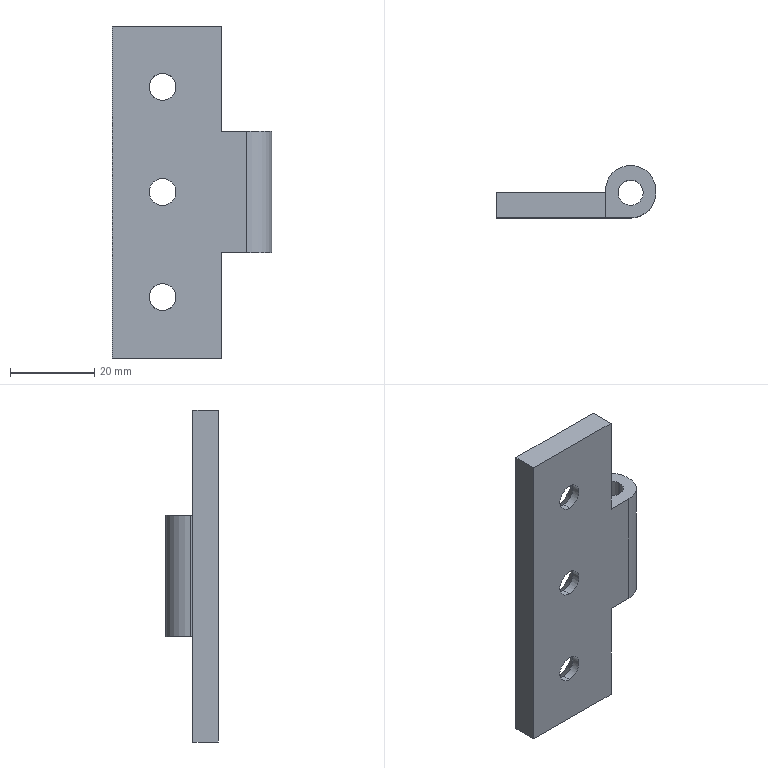Part | SolidWorks | features BaseBody 1 | 1 solid | 27 faces | box 38 x 12.5 x 79 mm | volume 13919 mm3 | plane 11 | cylinder 10 | cone 6 | commonest cylinder face diameters 6.4 x6 6 x2 12 x2
STEP:
#1=CARTESIAN_POINT('',(-43.,1552.,1081.7));
#2=VERTEX_POINT('',#1);
#3=CARTESIAN_POINT('',(-43.,1552.,1075.3));
#4=VERTEX_POINT('',#3);
#5=CARTESIAN_POINT('',(-43.,1552.,1078.5));
#6=DIRECTION('',(0.,-1.,0.));
#7=DIRECTION('',(0.,0.,1.));
#8=AXIS2_PLACEMENT_3D('',#5,#6,#7);
#9=CIRCLE('',#8,3.2);
#10=EDGE_CURVE('',#2,#4,#9,.T.);
#11=ORIENTED_EDGE('',*,*,#10,.T.);
#12=CARTESIAN_POINT('',(-43.,1556.,1071.3));
#13=VERTEX_POINT('',#12);
#14=CARTESIAN_POINT('',(-43.,1552.,1075.3));
#15=DIRECTION('',(0.,0.7071,-0.7071));
#16=VECTOR('',#15,1000.);
#17=LINE('',#14,#16);
#18=EDGE_CURVE('',#4,#13,#17,.T.);
#19=ORIENTED_EDGE('',*,*,#18,.T.);
#20=CARTESIAN_POINT('',(-43.,1556.,1085.7));
#21=VERTEX_POINT('',#20);
#22=CARTESIAN_POINT('',(-43.,1556.,1078.5));
#23=DIRECTION('',(0.,-1.,0.));
#24=DIRECTION('',(0.,0.,1.));
#25=AXIS2_PLACEMENT_3D('',#22,#23,#24);
#26=CIRCLE('',#25,7.2);
#27=EDGE_CURVE('',#21,#13,#26,.T.);
#28=ORIENTED_EDGE('',*,*,#27,.F.);
#29=CARTESIAN_POINT('',(-43.,1552.,1081.7));
#30=DIRECTION('',(0.,0.7071,0.7071));
#31=VECTOR('',#30,1000.);
#32=LINE('',#29,#31);
#33=EDGE_CURVE('',#2,#21,#32,.T.);
#34=ORIENTED_EDGE('',*,*,#33,.F.);
#35=EDGE_LOOP('',(#11,#19,#28,#34));
#36=FACE_OUTER_BOUND('',#35,.T.);
#37=CARTESIAN_POINT('',(-43.,1552.,1078.5));
#38=DIRECTION('',(0.,1.,0.));
#39=DIRECTION('',(0.,0.,1.));
#40=AXIS2_PLACEMENT_3D('',#37,#38,#39);
#41=CONICAL_SURFACE('',#40,3.2,0.7854);
#42=ADVANCED_FACE('',(#36),#41,.F.);
#43=CARTESIAN_POINT('',(-43.,1552.,1050.3));
#44=VERTEX_POINT('',#43);
#45=CARTESIAN_POINT('',(-39.8,1552.,1053.5));
#46=VERTEX_POINT('',#45);
#47=CARTESIAN_POINT('',(-43.,1552.,1053.5));
#48=DIRECTION('',(0.,-1.,0.));
#49=DIRECTION('',(0.,0.,1.));
#50=AXIS2_PLACEMENT_3D('',#47,#48,#49);
#51=CIRCLE('',#50,3.2);
#52=EDGE_CURVE('',#44,#46,#51,.T.);
#53=ORIENTED_EDGE('',*,*,#52,.T.);
#54=CARTESIAN_POINT('',(-35.8,1556.,1053.5));
#55=VERTEX_POINT('',#54);
#56=CARTESIAN_POINT('',(-39.8,1552.,1053.5));
#57=DIRECTION('',(0.7071,0.7071,0.));
#58=VECTOR('',#57,1000.);
#59=LINE('',#56,#58);
#60=EDGE_CURVE('',#46,#55,#59,.T.);
#61=ORIENTED_EDGE('',*,*,#60,.T.);
#62=CARTESIAN_POINT('',(-50.2,1556.,1053.5));
#63=VERTEX_POINT('',#62);
#64=CARTESIAN_POINT('',(-43.,1556.,1053.5));
#65=DIRECTION('',(0.,-1.,0.));
#66=DIRECTION('',(-1.,0.,0.));
#67=AXIS2_PLACEMENT_3D('',#64,#65,#66);
#68=CIRCLE('',#67,7.2);
#69=EDGE_CURVE('',#63,#55,#68,.T.);
#70=ORIENTED_EDGE('',*,*,#69,.F.);
#71=CARTESIAN_POINT('',(-46.2,1552.,1053.5));
#72=VERTEX_POINT('',#71);
#73=CARTESIAN_POINT('',(-46.2,1552.,1053.5));
#74=DIRECTION('',(-0.7071,0.7071,0.));
#75=VECTOR('',#74,1000.);
#76=LINE('',#73,#75);
#77=EDGE_CURVE('',#72,#63,#76,.T.);
#78=ORIENTED_EDGE('',*,*,#77,.F.);
#79=CARTESIAN_POINT('',(-43.,1552.,1053.5));
#80=DIRECTION('',(0.,-1.,0.));
#81=DIRECTION('',(0.,0.,1.));
#82=AXIS2_PLACEMENT_3D('',#79,#80,#81);
#83=CIRCLE('',#82,3.2);
#84=EDGE_CURVE('',#72,#44,#83,.T.);
#85=ORIENTED_EDGE('',*,*,#84,.T.);
#86=EDGE_LOOP('',(#53,#61,#70,#78,#85));
#87=FACE_OUTER_BOUND('',#86,.T.);
#88=CARTESIAN_POINT('',(-43.,1552.,1053.5));
#89=DIRECTION('',(0.,1.,0.));
#90=DIRECTION('',(-1.,0.,0.));
#91=AXIS2_PLACEMENT_3D('',#88,#89,#90);
#92=CONICAL_SURFACE('',#91,3.2,0.7854);
#93=ADVANCED_FACE('',(#87),#92,.F.);
#94=CARTESIAN_POINT('',(-43.,1552.,1100.3));
#95=VERTEX_POINT('',#94);
#96=CARTESIAN_POINT('',(-39.8,1552.,1103.5));
#97=VERTEX_POINT('',#96);
#98=CARTESIAN_POINT('',(-43.,1552.,1103.5));
#99=DIRECTION('',(0.,-1.,0.));
#100=DIRECTION('',(0.,0.,1.));
#101=AXIS2_PLACEMENT_3D('',#98,#99,#100);
#102=CIRCLE('',#101,3.2);
#103=EDGE_CURVE('',#95,#97,#102,.T.);
#104=ORIENTED_EDGE('',*,*,#103,.T.);
#105=CARTESIAN_POINT('',(-35.8,1556.,1103.5));
#106=VERTEX_POINT('',#105);
#107=CARTESIAN_POINT('',(-39.8,1552.,1103.5));
#108=DIRECTION('',(0.7071,0.7071,0.));
#109=VECTOR('',#108,1000.);
#110=LINE('',#107,#109);
#111=EDGE_CURVE('',#97,#106,#110,.T.);
#112=ORIENTED_EDGE('',*,*,#111,.T.);
#113=CARTESIAN_POINT('',(-50.2,1556.,1103.5));
#114=VERTEX_POINT('',#113);
#115=CARTESIAN_POINT('',(-43.,1556.,1103.5));
#116=DIRECTION('',(0.,-1.,0.));
#117=DIRECTION('',(-1.,0.,0.));
#118=AXIS2_PLACEMENT_3D('',#115,#116,#117);
#119=CIRCLE('',#118,7.2);
#120=EDGE_CURVE('',#114,#106,#119,.T.);
#121=ORIENTED_EDGE('',*,*,#120,.F.);
#122=CARTESIAN_POINT('',(-46.2,1552.,1103.5));
#123=VERTEX_POINT('',#122);
#124=CARTESIAN_POINT('',(-46.2,1552.,1103.5));
#125=DIRECTION('',(-0.7071,0.7071,0.));
#126=VECTOR('',#125,1000.);
#127=LINE('',#124,#126);
#128=EDGE_CURVE('',#123,#114,#127,.T.);
#129=ORIENTED_EDGE('',*,*,#128,.F.);
#130=CARTESIAN_POINT('',(-43.,1552.,1103.5));
#131=DIRECTION('',(0.,-1.,0.));
#132=DIRECTION('',(0.,0.,1.));
#133=AXIS2_PLACEMENT_3D('',#130,#131,#132);
#134=CIRCLE('',#133,3.2);
#135=EDGE_CURVE('',#123,#95,#134,.T.);
#136=ORIENTED_EDGE('',*,*,#135,.T.);
#137=EDGE_LOOP('',(#104,#112,#121,#129,#136));
#138=FACE_OUTER_BOUND('',#137,.T.);
#139=CARTESIAN_POINT('',(-43.,1552.,1103.5));
#140=DIRECTION('',(0.,1.,0.));
#141=DIRECTION('',(-1.,0.,0.));
#142=AXIS2_PLACEMENT_3D('',#139,#140,#141);
#143=CONICAL_SURFACE('',#142,3.2,0.7854);
#144=ADVANCED_FACE('',(#138),#143,.F.);
#145=CARTESIAN_POINT('',(-43.,1550.,1050.3));
#146=VERTEX_POINT('',#145);
#147=CARTESIAN_POINT('',(-43.,1550.,1056.7));
#148=VERTEX_POINT('',#147);
#149=CARTESIAN_POINT('',(-43.,1550.,1053.5));
#150=DIRECTION('',(0.,1.,0.));
#151=DIRECTION('',(0.,0.,1.));
#152=AXIS2_PLACEMENT_3D('',#149,#150,#151);
#153=CIRCLE('',#152,3.2);
#154=EDGE_CURVE('',#146,#148,#153,.T.);
#155=ORIENTED_EDGE('',*,*,#154,.F.);
#156=CARTESIAN_POINT('',(-43.,1550.,1050.3));
#157=DIRECTION('',(0.,1.,0.));
#158=VECTOR('',#157,1000.);
#159=LINE('',#156,#158);
#160=EDGE_CURVE('',#146,#44,#159,.T.);
#161=ORIENTED_EDGE('',*,*,#160,.T.);
#162=ORIENTED_EDGE('',*,*,#84,.F.);
#163=CARTESIAN_POINT('',(-43.,1552.,1056.7));
#164=VERTEX_POINT('',#163);
#165=CARTESIAN_POINT('',(-43.,1552.,1053.5));
#166=DIRECTION('',(0.,-1.,0.));
#167=DIRECTION('',(0.,0.,1.));
#168=AXIS2_PLACEMENT_3D('',#165,#166,#167);
#169=CIRCLE('',#168,3.2);
#170=EDGE_CURVE('',#164,#72,#169,.T.);
#171=ORIENTED_EDGE('',*,*,#170,.F.);
#172=CARTESIAN_POINT('',(-43.,1550.,1056.7));
#173=DIRECTION('',(0.,1.,0.));
#174=VECTOR('',#173,1000.);
#175=LINE('',#172,#174);
#176=EDGE_CURVE('',#148,#164,#175,.T.);
#177=ORIENTED_EDGE('',*,*,#176,.F.);
#178=EDGE_LOOP('',(#155,#161,#162,#171,#177));
#179=FACE_OUTER_BOUND('',#178,.T.);
#180=CARTESIAN_POINT('',(-43.,1550.,1053.5));
#181=DIRECTION('',(0.,1.,0.));
#182=DIRECTION('',(0.,0.,1.));
#183=AXIS2_PLACEMENT_3D('',#180,#181,#182);
#184=CYLINDRICAL_SURFACE('',#183,3.2);
#185=ADVANCED_FACE('',(#179),#184,.F.);
#186=CARTESIAN_POINT('',(-43.,1550.,1075.3));
#187=VERTEX_POINT('',#186);
#188=CARTESIAN_POINT('',(-43.,1550.,1081.7));
#189=VERTEX_POINT('',#188);
#190=CARTESIAN_POINT('',(-43.,1550.,1078.5));
#191=DIRECTION('',(0.,1.,0.));
#192=DIRECTION('',(0.,0.,1.));
#193=AXIS2_PLACEMENT_3D('',#190,#191,#192);
#194=CIRCLE('',#193,3.2);
#195=EDGE_CURVE('',#187,#189,#194,.T.);
#196=ORIENTED_EDGE('',*,*,#195,.F.);
#197=CARTESIAN_POINT('',(-43.,1550.,1075.3));
#198=DIRECTION('',(0.,1.,0.));
#199=VECTOR('',#198,1000.);
#200=LINE('',#197,#199);
#201=EDGE_CURVE('',#187,#4,#200,.T.);
#202=ORIENTED_EDGE('',*,*,#201,.T.);
#203=ORIENTED_EDGE('',*,*,#10,.F.);
#204=CARTESIAN_POINT('',(-43.,1550.,1081.7));
#205=DIRECTION('',(0.,1.,0.));
#206=VECTOR('',#205,1000.);
#207=LINE('',#204,#206);
#208=EDGE_CURVE('',#189,#2,#207,.T.);
#209=ORIENTED_EDGE('',*,*,#208,.F.);
#210=EDGE_LOOP('',(#196,#202,#203,#209));
#211=FACE_OUTER_BOUND('',#210,.T.);
#212=CARTESIAN_POINT('',(-43.,1550.,1078.5));
#213=DIRECTION('',(0.,1.,0.));
#214=DIRECTION('',(0.,0.,1.));
#215=AXIS2_PLACEMENT_3D('',#212,#213,#214);
#216=CYLINDRICAL_SURFACE('',#215,3.2);
#217=ADVANCED_FACE('',(#211),#216,.F.);
#218=CARTESIAN_POINT('',(-43.,1550.,1100.3));
#219=VERTEX_POINT('',#218);
#220=CARTESIAN_POINT('',(-43.,1550.,1106.7));
#221=VERTEX_POINT('',#220);
#222=CARTESIAN_POINT('',(-43.,1550.,1103.5));
#223=DIRECTION('',(0.,1.,0.));
#224=DIRECTION('',(0.,0.,1.));
#225=AXIS2_PLACEMENT_3D('',#222,#223,#224);
#226=CIRCLE('',#225,3.2);
#227=EDGE_CURVE('',#219,#221,#226,.T.);
#228=ORIENTED_EDGE('',*,*,#227,.F.);
#229=CARTESIAN_POINT('',(-43.,1550.,1100.3));
#230=DIRECTION('',(0.,1.,0.));
#231=VECTOR('',#230,1000.);
#232=LINE('',#229,#231);
#233=EDGE_CURVE('',#219,#95,#232,.T.);
#234=ORIENTED_EDGE('',*,*,#233,.T.);
#235=ORIENTED_EDGE('',*,*,#135,.F.);
#236=CARTESIAN_POINT('',(-43.,1552.,1106.7));
#237=VERTEX_POINT('',#236);
#238=CARTESIAN_POINT('',(-43.,1552.,1103.5));
#239=DIRECTION('',(0.,-1.,0.));
#240=DIRECTION('',(0.,0.,1.));
#241=AXIS2_PLACEMENT_3D('',#238,#239,#240);
#242=CIRCLE('',#241,3.2);
#243=EDGE_CURVE('',#237,#123,#242,.T.);
#244=ORIENTED_EDGE('',*,*,#243,.F.);
#245=CARTESIAN_POINT('',(-43.,1550.,1106.7));
#246=DIRECTION('',(0.,1.,0.));
#247=VECTOR('',#246,1000.);
#248=LINE('',#245,#247);
#249=EDGE_CURVE('',#221,#237,#248,.T.);
#250=ORIENTED_EDGE('',*,*,#249,.F.);
#251=EDGE_LOOP('',(#228,#234,#235,#244,#250));
#252=FACE_OUTER_BOUND('',#251,.T.);
#253=CARTESIAN_POINT('',(-43.,1550.,1103.5));
#254=DIRECTION('',(0.,1.,0.));
#255=DIRECTION('',(0.,0.,1.));
#256=AXIS2_PLACEMENT_3D('',#253,#254,#255);
#257=CYLINDRICAL_SURFACE('',#256,3.2);
#258=ADVANCED_FACE('',(#252),#257,.F.);
#259=CARTESIAN_POINT('',(-26.,1556.,1093.));
#260=VERTEX_POINT('',#259);
#261=CARTESIAN_POINT('',(-20.,1556.,1093.));
#262=VERTEX_POINT('',#261);
#263=CARTESIAN_POINT('',(-23.,1556.,1093.));
#264=DIRECTION('',(0.,0.,1.));
#265=DIRECTION('',(-1.,0.,0.));
#266=AXIS2_PLACEMENT_3D('',#263,#264,#265);
#267=CIRCLE('',#266,3.);
#268=EDGE_CURVE('',#260,#262,#267,.T.);
#269=ORIENTED_EDGE('',*,*,#268,.T.);
#270=CARTESIAN_POINT('',(-20.,1556.,1064.));
#271=VERTEX_POINT('',#270);
#272=CARTESIAN_POINT('',(-20.,1556.,1093.));
#273=DIRECTION('',(0.,0.,-1.));
#274=VECTOR('',#273,1000.);
#275=LINE('',#272,#274);
#276=EDGE_CURVE('',#262,#271,#275,.T.);
#277=ORIENTED_EDGE('',*,*,#276,.T.);
#278=CARTESIAN_POINT('',(-26.,1556.,1064.));
#279=VERTEX_POINT('',#278);
#280=CARTESIAN_POINT('',(-23.,1556.,1064.));
#281=DIRECTION('',(0.,0.,-1.));
#282=DIRECTION('',(-1.,0.,0.));
#283=AXIS2_PLACEMENT_3D('',#280,#281,#282);
#284=CIRCLE('',#283,3.);
#285=EDGE_CURVE('',#271,#279,#284,.T.);
#286=ORIENTED_EDGE('',*,*,#285,.T.);
#287=CARTESIAN_POINT('',(-26.,1556.,1093.));
#288=DIRECTION('',(0.,0.,-1.));
#289=VECTOR('',#288,1000.);
#290=LINE('',#287,#289);
#291=EDGE_CURVE('',#260,#279,#290,.T.);
#292=ORIENTED_EDGE('',*,*,#291,.F.);
#293=EDGE_LOOP('',(#269,#277,#286,#292));
#294=FACE_OUTER_BOUND('',#293,.T.);
#295=CARTESIAN_POINT('',(-23.,1556.,1093.));
#296=DIRECTION('',(0.,0.,-1.));
#297=DIRECTION('',(-1.,0.,0.));
#298=AXIS2_PLACEMENT_3D('',#295,#296,#297);
#299=CYLINDRICAL_SURFACE('',#298,3.);
#300=ADVANCED_FACE('',(#294),#299,.F.);
#301=CARTESIAN_POINT('',(-55.,1550.,1118.));
#302=VERTEX_POINT('',#301);
#303=CARTESIAN_POINT('',(-55.,1556.,1118.));
#304=VERTEX_POINT('',#303);
#305=CARTESIAN_POINT('',(-55.,1553.,1118.));
#306=DIRECTION('',(0.,1.,0.));
#307=VECTOR('',#306,1000.);
#308=LINE('',#305,#307);
#309=EDGE_CURVE('',#302,#304,#308,.T.);
#310=ORIENTED_EDGE('',*,*,#309,.F.);
#311=CARTESIAN_POINT('',(-29.,1550.,1118.));
#312=VERTEX_POINT('',#311);
#313=CARTESIAN_POINT('',(-42.,1550.,1118.));
#314=DIRECTION('',(-1.,0.,0.));
#315=VECTOR('',#314,1000.);
#316=LINE('',#313,#315);
#317=EDGE_CURVE('',#312,#302,#316,.T.);
#318=ORIENTED_EDGE('',*,*,#317,.F.);
#319=CARTESIAN_POINT('',(-29.,1556.,1118.));
#320=VERTEX_POINT('',#319);
#321=CARTESIAN_POINT('',(-29.,1553.,1118.));
#322=DIRECTION('',(0.,-1.,0.));
#323=VECTOR('',#322,1000.);
#324=LINE('',#321,#323);
#325=EDGE_CURVE('',#320,#312,#324,.T.);
#326=ORIENTED_EDGE('',*,*,#325,.F.);
#327=CARTESIAN_POINT('',(-42.,1556.,1118.));
#328=DIRECTION('',(1.,0.,0.));
#329=VECTOR('',#328,1000.);
#330=LINE('',#327,#329);
#331=EDGE_CURVE('',#304,#320,#330,.T.);
#332=ORIENTED_EDGE('',*,*,#331,.F.);
#333=EDGE_LOOP('',(#310,#318,#326,#332));
#334=FACE_OUTER_BOUND('',#333,.T.);
#335=CARTESIAN_POINT('',(-28.48,1549.88,1118.));
#336=DIRECTION('',(0.,0.,-1.));
#337=DIRECTION('',(-1.,0.,0.));
#338=AXIS2_PLACEMENT_3D('',#335,#336,#337);
#339=PLANE('',#338);
#340=ADVANCED_FACE('',(#334),#339,.F.);
#341=ORIENTED_EDGE('',*,*,#27,.T.);
#342=CARTESIAN_POINT('',(-43.,1556.,1078.5));
#343=DIRECTION('',(0.,-1.,0.));
#344=DIRECTION('',(0.,0.,1.));
#345=AXIS2_PLACEMENT_3D('',#342,#343,#344);
#346=CIRCLE('',#345,7.2);
#347=EDGE_CURVE('',#13,#21,#346,.T.);
#348=ORIENTED_EDGE('',*,*,#347,.T.);
#349=EDGE_LOOP('',(#341,#348));
#350=FACE_BOUND('',#349,.T.);
#351=ORIENTED_EDGE('',*,*,#69,.T.);
#352=CARTESIAN_POINT('',(-43.,1556.,1053.5));
#353=DIRECTION('',(0.,-1.,0.));
#354=DIRECTION('',(-1.,0.,0.));
#355=AXIS2_PLACEMENT_3D('',#352,#353,#354);
#356=CIRCLE('',#355,7.2);
#357=EDGE_CURVE('',#55,#63,#356,.T.);
#358=ORIENTED_EDGE('',*,*,#357,.T.);
#359=EDGE_LOOP('',(#351,#358));
#360=FACE_BOUND('',#359,.T.);
#361=ORIENTED_EDGE('',*,*,#120,.T.);
#362=CARTESIAN_POINT('',(-43.,1556.,1103.5));
#363=DIRECTION('',(0.,-1.,0.));
#364=DIRECTION('',(-1.,0.,0.));
#365=AXIS2_PLACEMENT_3D('',#362,#363,#364);
#366=CIRCLE('',#365,7.2);
#367=EDGE_CURVE('',#106,#114,#366,.T.);
#368=ORIENTED_EDGE('',*,*,#367,.T.);
#369=EDGE_LOOP('',(#361,#368));
#370=FACE_BOUND('',#369,.T.);
#371=ORIENTED_EDGE('',*,*,#331,.T.);
#372=CARTESIAN_POINT('',(-29.,1556.,1093.));
#373=VERTEX_POINT('',#372);
#374=CARTESIAN_POINT('',(-29.,1556.,1078.5));
#375=DIRECTION('',(0.,0.,-1.));
#376=VECTOR('',#375,1000.);
#377=LINE('',#374,#376);
#378=EDGE_CURVE('',#320,#373,#377,.T.);
#379=ORIENTED_EDGE('',*,*,#378,.T.);
#380=CARTESIAN_POINT('',(-29.,1556.,1064.));
#381=VERTEX_POINT('',#380);
#382=CARTESIAN_POINT('',(-29.,1556.,1078.5));
#383=DIRECTION('',(0.,0.,-1.));
#384=VECTOR('',#383,1000.);
#385=LINE('',#382,#384);
#386=EDGE_CURVE('',#373,#381,#385,.T.);
#387=ORIENTED_EDGE('',*,*,#386,.T.);
#388=CARTESIAN_POINT('',(-29.,1556.,1039.));
#389=VERTEX_POINT('',#388);
#390=CARTESIAN_POINT('',(-29.,1556.,1078.5));
#391=DIRECTION('',(0.,0.,-1.));
#392=VECTOR('',#391,1000.);
#393=LINE('',#390,#392);
#394=EDGE_CURVE('',#381,#389,#393,.T.);
#395=ORIENTED_EDGE('',*,*,#394,.T.);
#396=CARTESIAN_POINT('',(-55.,1556.,1039.));
#397=VERTEX_POINT('',#396);
#398=CARTESIAN_POINT('',(-42.,1556.,1039.));
#399=DIRECTION('',(-1.,0.,0.));
#400=VECTOR('',#399,1000.);
#401=LINE('',#398,#400);
#402=EDGE_CURVE('',#389,#397,#401,.T.);
#403=ORIENTED_EDGE('',*,*,#402,.T.);
#404=CARTESIAN_POINT('',(-55.,1556.,1078.5));
#405=DIRECTION('',(0.,0.,1.));
#406=VECTOR('',#405,1000.);
#407=LINE('',#404,#406);
#408=EDGE_CURVE('',#397,#304,#407,.T.);
#409=ORIENTED_EDGE('',*,*,#408,.T.);
#410=EDGE_LOOP('',(#371,#379,#387,#395,#403,#409));
#411=FACE_OUTER_BOUND('',#410,.T.);
#412=CARTESIAN_POINT('',(-55.52,1556.,1119.58));
#413=DIRECTION('',(0.,1.,0.));
#414=DIRECTION('',(1.,0.,0.));
#415=AXIS2_PLACEMENT_3D('',#412,#413,#414);
#416=PLANE('',#415);
#417=ADVANCED_FACE('',(#350,#360,#370,#411),#416,.T.);
#418=CARTESIAN_POINT('',(-55.,1550.,1039.));
#419=VERTEX_POINT('',#418);
#420=CARTESIAN_POINT('',(-55.,1553.,1039.));
#421=DIRECTION('',(0.,-1.,0.));
#422=VECTOR('',#421,1000.);
#423=LINE('',#420,#422);
#424=EDGE_CURVE('',#397,#419,#423,.T.);
#425=ORIENTED_EDGE('',*,*,#424,.T.);
#426=CARTESIAN_POINT('',(-55.,1550.,1078.5));
#427=DIRECTION('',(0.,0.,1.));
#428=VECTOR('',#427,1000.);
#429=LINE('',#426,#428);
#430=EDGE_CURVE('',#419,#302,#429,.T.);
#431=ORIENTED_EDGE('',*,*,#430,.T.);
#432=ORIENTED_EDGE('',*,*,#309,.T.);
#433=ORIENTED_EDGE('',*,*,#408,.F.);
#434=EDGE_LOOP('',(#425,#431,#432,#433));
#435=FACE_OUTER_BOUND('',#434,.T.);
#436=CARTESIAN_POINT('',(-55.,1549.88,1119.58));
#437=DIRECTION('',(-1.,0.,0.));
#438=DIRECTION('',(0.,1.,0.));
#439=AXIS2_PLACEMENT_3D('',#436,#437,#438);
#440=PLANE('',#439);
#441=ADVANCED_FACE('',(#435),#440,.T.);
#442=CARTESIAN_POINT('',(-43.,1550.,1053.5));
#443=DIRECTION('',(0.,1.,0.));
#444=DIRECTION('',(0.,0.,1.));
#445=AXIS2_PLACEMENT_3D('',#442,#443,#444);
#446=CIRCLE('',#445,3.2);
#447=EDGE_CURVE('',#148,#146,#446,.T.);
#448=ORIENTED_EDGE('',*,*,#447,.T.);
#449=ORIENTED_EDGE('',*,*,#154,.T.);
#450=EDGE_LOOP('',(#448,#449));
#451=FACE_BOUND('',#450,.T.);
#452=CARTESIAN_POINT('',(-43.,1550.,1078.5));
#453=DIRECTION('',(0.,1.,0.));
#454=DIRECTION('',(0.,0.,1.));
#455=AXIS2_PLACEMENT_3D('',#452,#453,#454);
#456=CIRCLE('',#455,3.2);
#457=EDGE_CURVE('',#189,#187,#456,.T.);
#458=ORIENTED_EDGE('',*,*,#457,.T.);
#459=ORIENTED_EDGE('',*,*,#195,.T.);
#460=EDGE_LOOP('',(#458,#459));
#461=FACE_BOUND('',#460,.T.);
#462=CARTESIAN_POINT('',(-43.,1550.,1103.5));
#463=DIRECTION('',(0.,1.,0.));
#464=DIRECTION('',(0.,0.,1.));
#465=AXIS2_PLACEMENT_3D('',#462,#463,#464);
#466=CIRCLE('',#465,3.2);
#467=EDGE_CURVE('',#221,#219,#466,.T.);
#468=ORIENTED_EDGE('',*,*,#467,.T.);
#469=ORIENTED_EDGE('',*,*,#227,.T.);
#470=EDGE_LOOP('',(#468,#469));
#471=FACE_BOUND('',#470,.T.);
#472=CARTESIAN_POINT('',(-29.,1550.,1039.));
#473=VERTEX_POINT('',#472);
#474=CARTESIAN_POINT('',(-29.,1550.,1064.));
#475=VERTEX_POINT('',#474);
#476=CARTESIAN_POINT('',(-29.,1550.,1078.5));
#477=DIRECTION('',(0.,0.,1.));
#478=VECTOR('',#477,1000.);
#479=LINE('',#476,#478);
#480=EDGE_CURVE('',#473,#475,#479,.T.);
#481=ORIENTED_EDGE('',*,*,#480,.T.);
#482=CARTESIAN_POINT('',(-23.,1550.,1064.));
#483=VERTEX_POINT('',#482);
#484=CARTESIAN_POINT('',(-39.,1550.,1064.));
#485=DIRECTION('',(1.,0.,0.));
#486=VECTOR('',#485,1000.);
#487=LINE('',#484,#486);
#488=EDGE_CURVE('',#475,#483,#487,.T.);
#489=ORIENTED_EDGE('',*,*,#488,.T.);
#490=CARTESIAN_POINT('',(-23.,1550.,1093.));
#491=VERTEX_POINT('',#490);
#492=CARTESIAN_POINT('',(-23.,1550.,1078.5));
#493=DIRECTION('',(0.,0.,1.));
#494=VECTOR('',#493,1000.);
#495=LINE('',#492,#494);
#496=EDGE_CURVE('',#483,#491,#495,.T.);
#497=ORIENTED_EDGE('',*,*,#496,.T.);
#498=CARTESIAN_POINT('',(-29.,1550.,1093.));
#499=VERTEX_POINT('',#498);
#500=CARTESIAN_POINT('',(-39.,1550.,1093.));
#501=DIRECTION('',(-1.,0.,0.));
#502=VECTOR('',#501,1000.);
#503=LINE('',#500,#502);
#504=EDGE_CURVE('',#491,#499,#503,.T.);
#505=ORIENTED_EDGE('',*,*,#504,.T.);
#506=CARTESIAN_POINT('',(-29.,1550.,1078.5));
#507=DIRECTION('',(0.,0.,1.));
#508=VECTOR('',#507,1000.);
#509=LINE('',#506,#508);
#510=EDGE_CURVE('',#499,#312,#509,.T.);
#511=ORIENTED_EDGE('',*,*,#510,.T.);
#512=ORIENTED_EDGE('',*,*,#317,.T.);
#513=ORIENTED_EDGE('',*,*,#430,.F.);
#514=CARTESIAN_POINT('',(-39.,1550.,1039.));
#515=DIRECTION('',(1.,0.,0.));
#516=VECTOR('',#515,1000.);
#517=LINE('',#514,#516);
#518=EDGE_CURVE('',#419,#473,#517,.T.);
#519=ORIENTED_EDGE('',*,*,#518,.T.);
#520=EDGE_LOOP('',(#481,#489,#497,#505,#511,#512,#513,#519));
#521=FACE_OUTER_BOUND('',#520,.T.);
#522=CARTESIAN_POINT('',(-22.36,1550.,1119.58));
#523=DIRECTION('',(0.,-1.,0.));
#524=DIRECTION('',(-1.,0.,0.));
#525=AXIS2_PLACEMENT_3D('',#522,#523,#524);
#526=PLANE('',#525);
#527=ADVANCED_FACE('',(#451,#461,#471,#521),#526,.T.);
#528=CARTESIAN_POINT('',(-29.,1553.,1093.));
#529=DIRECTION('',(0.,-1.,0.));
#530=VECTOR('',#529,1000.);
#531=LINE('',#528,#530);
#532=EDGE_CURVE('',#373,#499,#531,.T.);
#533=ORIENTED_EDGE('',*,*,#532,.F.);
#534=ORIENTED_EDGE('',*,*,#378,.F.);
#535=ORIENTED_EDGE('',*,*,#325,.T.);
#536=ORIENTED_EDGE('',*,*,#510,.F.);
#537=EDGE_LOOP('',(#533,#534,#535,#536));
#538=FACE_OUTER_BOUND('',#537,.T.);
#539=CARTESIAN_POINT('',(-29.,1549.88,1092.5));
#540=DIRECTION('',(-1.,0.,0.));
#541=DIRECTION('',(0.,0.,1.));
#542=AXIS2_PLACEMENT_3D('',#539,#540,#541);
#543=PLANE('',#542);
#544=ADVANCED_FACE('',(#538),#543,.F.);
#545=ORIENTED_EDGE('',*,*,#18,.F.);
#546=CARTESIAN_POINT('',(-43.,1552.,1078.5));
#547=DIRECTION('',(0.,-1.,0.));
#548=DIRECTION('',(0.,0.,1.));
#549=AXIS2_PLACEMENT_3D('',#546,#547,#548);
#550=CIRCLE('',#549,3.2);
#551=EDGE_CURVE('',#4,#2,#550,.T.);
#552=ORIENTED_EDGE('',*,*,#551,.T.);
#553=ORIENTED_EDGE('',*,*,#33,.T.);
#554=ORIENTED_EDGE('',*,*,#347,.F.);
#555=EDGE_LOOP('',(#545,#552,#553,#554));
#556=FACE_OUTER_BOUND('',#555,.T.);
#557=CARTESIAN_POINT('',(-43.,1552.,1078.5));
#558=DIRECTION('',(0.,1.,0.));
#559=DIRECTION('',(0.,0.,1.));
#560=AXIS2_PLACEMENT_3D('',#557,#558,#559);
#561=CONICAL_SURFACE('',#560,3.2,0.7854);
#562=ADVANCED_FACE('',(#556),#561,.F.);
#563=ORIENTED_EDGE('',*,*,#60,.F.);
#564=CARTESIAN_POINT('',(-43.,1552.,1053.5));
#565=DIRECTION('',(0.,-1.,0.));
#566=DIRECTION('',(0.,0.,1.));
#567=AXIS2_PLACEMENT_3D('',#564,#565,#566);
#568=CIRCLE('',#567,3.2);
#569=EDGE_CURVE('',#46,#164,#568,.T.);
#570=ORIENTED_EDGE('',*,*,#569,.T.);
#571=ORIENTED_EDGE('',*,*,#170,.T.);
#572=ORIENTED_EDGE('',*,*,#77,.T.);
#573=ORIENTED_EDGE('',*,*,#357,.F.);
#574=EDGE_LOOP('',(#563,#570,#571,#572,#573));
#575=FACE_OUTER_BOUND('',#574,.T.);
#576=CARTESIAN_POINT('',(-43.,1552.,1053.5));
#577=DIRECTION('',(0.,1.,0.));
#578=DIRECTION('',(-1.,0.,0.));
#579=AXIS2_PLACEMENT_3D('',#576,#577,#578);
#580=CONICAL_SURFACE('',#579,3.2,0.7854);
#581=ADVANCED_FACE('',(#575),#580,.F.);
#582=ORIENTED_EDGE('',*,*,#111,.F.);
#583=CARTESIAN_POINT('',(-43.,1552.,1103.5));
#584=DIRECTION('',(0.,-1.,0.));
#585=DIRECTION('',(0.,0.,1.));
#586=AXIS2_PLACEMENT_3D('',#583,#584,#585);
#587=CIRCLE('',#586,3.2);
#588=EDGE_CURVE('',#97,#237,#587,.T.);
#589=ORIENTED_EDGE('',*,*,#588,.T.);
#590=ORIENTED_EDGE('',*,*,#243,.T.);
#591=ORIENTED_EDGE('',*,*,#128,.T.);
#592=ORIENTED_EDGE('',*,*,#367,.F.);
#593=EDGE_LOOP('',(#582,#589,#590,#591,#592));
#594=FACE_OUTER_BOUND('',#593,.T.);
#595=CARTESIAN_POINT('',(-43.,1552.,1103.5));
#596=DIRECTION('',(0.,1.,0.));
#597=DIRECTION('',(-1.,0.,0.));
#598=AXIS2_PLACEMENT_3D('',#595,#596,#597);
#599=CONICAL_SURFACE('',#598,3.2,0.7854);
#600=ADVANCED_FACE('',(#594),#599,.F.);
#601=ORIENTED_EDGE('',*,*,#424,.F.);
#602=ORIENTED_EDGE('',*,*,#402,.F.);
#603=CARTESIAN_POINT('',(-29.,1553.,1039.));
#604=DIRECTION('',(0.,-1.,0.));
#605=VECTOR('',#604,1000.);
#606=LINE('',#603,#605);
#607=EDGE_CURVE('',#389,#473,#606,.T.);
#608=ORIENTED_EDGE('',*,*,#607,.T.);
#609=ORIENTED_EDGE('',*,*,#518,.F.);
#610=EDGE_LOOP('',(#601,#602,#608,#609));
#611=FACE_OUTER_BOUND('',#610,.T.);
#612=CARTESIAN_POINT('',(-28.48,1549.88,1039.));
#613=DIRECTION('',(0.,0.,-1.));
#614=DIRECTION('',(-1.,0.,0.));
#615=AXIS2_PLACEMENT_3D('',#612,#613,#614);
#616=PLANE('',#615);
#617=ADVANCED_FACE('',(#611),#616,.T.);
#618=CARTESIAN_POINT('',(-29.,1553.,1064.));
#619=DIRECTION('',(0.,1.,0.));
#620=VECTOR('',#619,1000.);
#621=LINE('',#618,#620);
#622=EDGE_CURVE('',#475,#381,#621,.T.);
#623=ORIENTED_EDGE('',*,*,#622,.F.);
#624=ORIENTED_EDGE('',*,*,#480,.F.);
#625=ORIENTED_EDGE('',*,*,#607,.F.);
#626=ORIENTED_EDGE('',*,*,#394,.F.);
#627=EDGE_LOOP('',(#623,#624,#625,#626));
#628=FACE_OUTER_BOUND('',#627,.T.);
#629=CARTESIAN_POINT('',(-29.,1549.88,1038.5));
#630=DIRECTION('',(-1.,0.,0.));
#631=DIRECTION('',(0.,0.,1.));
#632=AXIS2_PLACEMENT_3D('',#629,#630,#631);
#633=PLANE('',#632);
#634=ADVANCED_FACE('',(#628),#633,.F.);
#635=ORIENTED_EDGE('',*,*,#386,.F.);
#636=CARTESIAN_POINT('',(-29.,1556.5,1093.));
#637=VERTEX_POINT('',#636);
#638=CARTESIAN_POINT('',(-29.,1556.25,1093.));
#639=DIRECTION('',(0.,1.,0.));
#640=VECTOR('',#639,1000.);
#641=LINE('',#638,#640);
#642=EDGE_CURVE('',#373,#637,#641,.T.);
#643=ORIENTED_EDGE('',*,*,#642,.T.);
#644=CARTESIAN_POINT('',(-29.,1556.5,1064.));
#645=VERTEX_POINT('',#644);
#646=CARTESIAN_POINT('',(-29.,1556.5,1078.5));
#647=DIRECTION('',(0.,0.,-1.));
#648=VECTOR('',#647,1000.);
#649=LINE('',#646,#648);
#650=EDGE_CURVE('',#637,#645,#649,.T.);
#651=ORIENTED_EDGE('',*,*,#650,.T.);
#652=CARTESIAN_POINT('',(-29.,1556.25,1064.));
#653=DIRECTION('',(0.,-1.,0.));
#654=VECTOR('',#653,1000.);
#655=LINE('',#652,#654);
#656=EDGE_CURVE('',#645,#381,#655,.T.);
#657=ORIENTED_EDGE('',*,*,#656,.T.);
#658=EDGE_LOOP('',(#635,#643,#651,#657));
#659=FACE_OUTER_BOUND('',#658,.T.);
#660=CARTESIAN_POINT('',(-29.,1555.894,1093.58));
#661=DIRECTION('',(-1.,0.,0.));
#662=DIRECTION('',(0.,1.,0.));
#663=AXIS2_PLACEMENT_3D('',#660,#661,#662);
#664=PLANE('',#663);
#665=ADVANCED_FACE('',(#659),#664,.T.);
#666=ORIENTED_EDGE('',*,*,#160,.F.);
#667=ORIENTED_EDGE('',*,*,#447,.F.);
#668=ORIENTED_EDGE('',*,*,#176,.T.);
#669=ORIENTED_EDGE('',*,*,#569,.F.);
#670=ORIENTED_EDGE('',*,*,#52,.F.);
#671=EDGE_LOOP('',(#666,#667,#668,#669,#670));
#672=FACE_OUTER_BOUND('',#671,.T.);
#673=CARTESIAN_POINT('',(-43.,1550.,1053.5));
#674=DIRECTION('',(0.,1.,0.));
#675=DIRECTION('',(0.,0.,1.));
#676=AXIS2_PLACEMENT_3D('',#673,#674,#675);
#677=CYLINDRICAL_SURFACE('',#676,3.2);
#678=ADVANCED_FACE('',(#672),#677,.F.);
#679=ORIENTED_EDGE('',*,*,#201,.F.);
#680=ORIENTED_EDGE('',*,*,#457,.F.);
#681=ORIENTED_EDGE('',*,*,#208,.T.);
#682=ORIENTED_EDGE('',*,*,#551,.F.);
#683=EDGE_LOOP('',(#679,#680,#681,#682));
#684=FACE_OUTER_BOUND('',#683,.T.);
#685=CARTESIAN_POINT('',(-43.,1550.,1078.5));
#686=DIRECTION('',(0.,1.,0.));
#687=DIRECTION('',(0.,0.,1.));
#688=AXIS2_PLACEMENT_3D('',#685,#686,#687);
#689=CYLINDRICAL_SURFACE('',#688,3.2);
#690=ADVANCED_FACE('',(#684),#689,.F.);
#691=ORIENTED_EDGE('',*,*,#233,.F.);
#692=ORIENTED_EDGE('',*,*,#467,.F.);
#693=ORIENTED_EDGE('',*,*,#249,.T.);
#694=ORIENTED_EDGE('',*,*,#588,.F.);
#695=ORIENTED_EDGE('',*,*,#103,.F.);
#696=EDGE_LOOP('',(#691,#692,#693,#694,#695));
#697=FACE_OUTER_BOUND('',#696,.T.);
#698=CARTESIAN_POINT('',(-43.,1550.,1103.5));
#699=DIRECTION('',(0.,1.,0.));
#700=DIRECTION('',(0.,0.,1.));
#701=AXIS2_PLACEMENT_3D('',#698,#699,#700);
#702=CYLINDRICAL_SURFACE('',#701,3.2);
#703=ADVANCED_FACE('',(#697),#702,.F.);
#704=CARTESIAN_POINT('',(-23.,1556.,1064.));
#705=DIRECTION('',(0.,0.,-1.));
#706=DIRECTION('',(-1.,0.,0.));
#707=AXIS2_PLACEMENT_3D('',#704,#705,#706);
#708=CIRCLE('',#707,3.);
#709=EDGE_CURVE('',#279,#271,#708,.T.);
#710=ORIENTED_EDGE('',*,*,#709,.F.);
#711=ORIENTED_EDGE('',*,*,#285,.F.);
#712=EDGE_LOOP('',(#710,#711));
#713=FACE_BOUND('',#712,.T.);
#714=CARTESIAN_POINT('',(-17.,1556.,1064.));
#715=VERTEX_POINT('',#714);
#716=CARTESIAN_POINT('',(-23.,1556.,1064.));
#717=DIRECTION('',(0.,0.,1.));
#718=DIRECTION('',(1.,0.,0.));
#719=AXIS2_PLACEMENT_3D('',#716,#717,#718);
#720=CIRCLE('',#719,6.);
#721=EDGE_CURVE('',#483,#715,#720,.T.);
#722=ORIENTED_EDGE('',*,*,#721,.F.);
#723=ORIENTED_EDGE('',*,*,#488,.F.);
#724=ORIENTED_EDGE('',*,*,#622,.T.);
#725=ORIENTED_EDGE('',*,*,#656,.F.);
#726=CARTESIAN_POINT('',(-17.,1556.5,1064.));
#727=VERTEX_POINT('',#726);
#728=CARTESIAN_POINT('',(-23.,1556.5,1064.));
#729=DIRECTION('',(0.,0.,1.));
#730=DIRECTION('',(1.,0.,0.));
#731=AXIS2_PLACEMENT_3D('',#728,#729,#730);
#732=CIRCLE('',#731,6.);
#733=EDGE_CURVE('',#727,#645,#732,.T.);
#734=ORIENTED_EDGE('',*,*,#733,.F.);
#735=CARTESIAN_POINT('',(-17.,1556.25,1064.));
#736=DIRECTION('',(0.,1.,0.));
#737=VECTOR('',#736,1000.);
#738=LINE('',#735,#737);
#739=EDGE_CURVE('',#715,#727,#738,.T.);
#740=ORIENTED_EDGE('',*,*,#739,.F.);
#741=EDGE_LOOP('',(#722,#723,#724,#725,#734,#740));
#742=FACE_OUTER_BOUND('',#741,.T.);
#743=CARTESIAN_POINT('',(-29.24,1549.75,1064.));
#744=DIRECTION('',(0.,0.,1.));
#745=DIRECTION('',(1.,0.,0.));
#746=AXIS2_PLACEMENT_3D('',#743,#744,#745);
#747=PLANE('',#746);
#748=ADVANCED_FACE('',(#713,#742),#747,.F.);
#749=ORIENTED_EDGE('',*,*,#268,.F.);
#750=CARTESIAN_POINT('',(-23.,1556.,1093.));
#751=DIRECTION('',(0.,0.,1.));
#752=DIRECTION('',(-1.,0.,0.));
#753=AXIS2_PLACEMENT_3D('',#750,#751,#752);
#754=CIRCLE('',#753,3.);
#755=EDGE_CURVE('',#262,#260,#754,.T.);
#756=ORIENTED_EDGE('',*,*,#755,.F.);
#757=EDGE_LOOP('',(#749,#756));
#758=FACE_BOUND('',#757,.T.);
#759=ORIENTED_EDGE('',*,*,#532,.T.);
#760=ORIENTED_EDGE('',*,*,#504,.F.);
#761=CARTESIAN_POINT('',(-17.,1556.,1093.));
#762=VERTEX_POINT('',#761);
#763=CARTESIAN_POINT('',(-23.,1556.,1093.));
#764=DIRECTION('',(0.,0.,-1.));
#765=DIRECTION('',(1.,0.,0.));
#766=AXIS2_PLACEMENT_3D('',#763,#764,#765);
#767=CIRCLE('',#766,6.);
#768=EDGE_CURVE('',#762,#491,#767,.T.);
#769=ORIENTED_EDGE('',*,*,#768,.F.);
#770=CARTESIAN_POINT('',(-17.,1556.5,1093.));
#771=VERTEX_POINT('',#770);
#772=CARTESIAN_POINT('',(-17.,1556.25,1093.));
#773=DIRECTION('',(0.,-1.,0.));
#774=VECTOR('',#773,1000.);
#775=LINE('',#772,#774);
#776=EDGE_CURVE('',#771,#762,#775,.T.);
#777=ORIENTED_EDGE('',*,*,#776,.F.);
#778=CARTESIAN_POINT('',(-23.,1556.5,1093.));
#779=DIRECTION('',(0.,0.,-1.));
#780=DIRECTION('',(1.,0.,0.));
#781=AXIS2_PLACEMENT_3D('',#778,#779,#780);
#782=CIRCLE('',#781,6.);
#783=EDGE_CURVE('',#637,#771,#782,.T.);
#784=ORIENTED_EDGE('',*,*,#783,.F.);
#785=ORIENTED_EDGE('',*,*,#642,.F.);
#786=EDGE_LOOP('',(#759,#760,#769,#777,#784,#785));
#787=FACE_OUTER_BOUND('',#786,.T.);
#788=CARTESIAN_POINT('',(-16.76,1549.75,1093.));
#789=DIRECTION('',(0.,0.,-1.));
#790=DIRECTION('',(-1.,0.,0.));
#791=AXIS2_PLACEMENT_3D('',#788,#789,#790);
#792=PLANE('',#791);
#793=ADVANCED_FACE('',(#758,#787),#792,.F.);
#794=ORIENTED_EDGE('',*,*,#721,.T.);
#795=CARTESIAN_POINT('',(-17.,1556.,1078.5));
#796=DIRECTION('',(0.,0.,-1.));
#797=VECTOR('',#796,1000.);
#798=LINE('',#795,#797);
#799=EDGE_CURVE('',#762,#715,#798,.T.);
#800=ORIENTED_EDGE('',*,*,#799,.F.);
#801=ORIENTED_EDGE('',*,*,#768,.T.);
#802=ORIENTED_EDGE('',*,*,#496,.F.);
#803=EDGE_LOOP('',(#794,#800,#801,#802));
#804=FACE_OUTER_BOUND('',#803,.T.);
#805=CARTESIAN_POINT('',(-23.,1556.,1064.));
#806=DIRECTION('',(0.,0.,1.));
#807=DIRECTION('',(1.,0.,0.));
#808=AXIS2_PLACEMENT_3D('',#805,#806,#807);
#809=CYLINDRICAL_SURFACE('',#808,6.);
#810=ADVANCED_FACE('',(#804),#809,.T.);
#811=ORIENTED_EDGE('',*,*,#783,.T.);
#812=CARTESIAN_POINT('',(-17.,1556.5,1078.5));
#813=DIRECTION('',(0.,0.,1.));
#814=VECTOR('',#813,1000.);
#815=LINE('',#812,#814);
#816=EDGE_CURVE('',#727,#771,#815,.T.);
#817=ORIENTED_EDGE('',*,*,#816,.F.);
#818=ORIENTED_EDGE('',*,*,#733,.T.);
#819=ORIENTED_EDGE('',*,*,#650,.F.);
#820=EDGE_LOOP('',(#811,#817,#818,#819));
#821=FACE_OUTER_BOUND('',#820,.T.);
#822=CARTESIAN_POINT('',(-23.,1556.5,1064.));
#823=DIRECTION('',(0.,0.,1.));
#824=DIRECTION('',(1.,0.,0.));
#825=AXIS2_PLACEMENT_3D('',#822,#823,#824);
#826=CYLINDRICAL_SURFACE('',#825,6.);
#827=ADVANCED_FACE('',(#821),#826,.T.);
#828=ORIENTED_EDGE('',*,*,#276,.F.);
#829=ORIENTED_EDGE('',*,*,#755,.T.);
#830=ORIENTED_EDGE('',*,*,#291,.T.);
#831=ORIENTED_EDGE('',*,*,#709,.T.);
#832=EDGE_LOOP('',(#828,#829,#830,#831));
#833=FACE_OUTER_BOUND('',#832,.T.);
#834=CARTESIAN_POINT('',(-23.,1556.,1093.));
#835=DIRECTION('',(0.,0.,-1.));
#836=DIRECTION('',(-1.,0.,0.));
#837=AXIS2_PLACEMENT_3D('',#834,#835,#836);
#838=CYLINDRICAL_SURFACE('',#837,3.);
#839=ADVANCED_FACE('',(#833),#838,.F.);
#840=ORIENTED_EDGE('',*,*,#799,.T.);
#841=ORIENTED_EDGE('',*,*,#739,.T.);
#842=ORIENTED_EDGE('',*,*,#816,.T.);
#843=ORIENTED_EDGE('',*,*,#776,.T.);
#844=EDGE_LOOP('',(#840,#841,#842,#843));
#845=FACE_OUTER_BOUND('',#844,.T.);
#846=CARTESIAN_POINT('',(-17.,1556.606,1093.58));
#847=DIRECTION('',(1.,0.,0.));
#848=DIRECTION('',(0.,-1.,0.));
#849=AXIS2_PLACEMENT_3D('',#846,#847,#848);
#850=PLANE('',#849);
#851=ADVANCED_FACE('',(#845),#850,.T.);
#852=CLOSED_SHELL('',(#42,#93,#144,#185,#217,#258,#300,#340,#417,#441,#527,#544,#562,#581,#600,#617,#634,#665,#678,#690,#703,#748,#793,#810,#827,#839,#851));
#853=MANIFOLD_SOLID_BREP('',#852);
#854=CARTESIAN_POINT('',(0.,0.,0.));
#855=DIRECTION('',(0.,0.,1.));
#856=DIRECTION('',(1.,0.,0.));
#857=AXIS2_PLACEMENT_3D('',#854,#855,#856);
#858=(LENGTH_UNIT()NAMED_UNIT(*)SI_UNIT(.MILLI.,.METRE.));
#859=UNCERTAINTY_MEASURE_WITH_UNIT(LENGTH_MEASURE(0.00001),#858,'','');
#860=(NAMED_UNIT(*)PLANE_ANGLE_UNIT()SI_UNIT($,.RADIAN.));
#861=(NAMED_UNIT(*)SI_UNIT($,.STERADIAN.)SOLID_ANGLE_UNIT());
#862=(GEOMETRIC_REPRESENTATION_CONTEXT(3)GLOBAL_UNCERTAINTY_ASSIGNED_CONTEXT((#859))GLOBAL_UNIT_ASSIGNED_CONTEXT((#858,#860,#861))REPRESENTATION_CONTEXT('',''));
#863=ADVANCED_BREP_SHAPE_REPRESENTATION('',(#853,#857),#862);